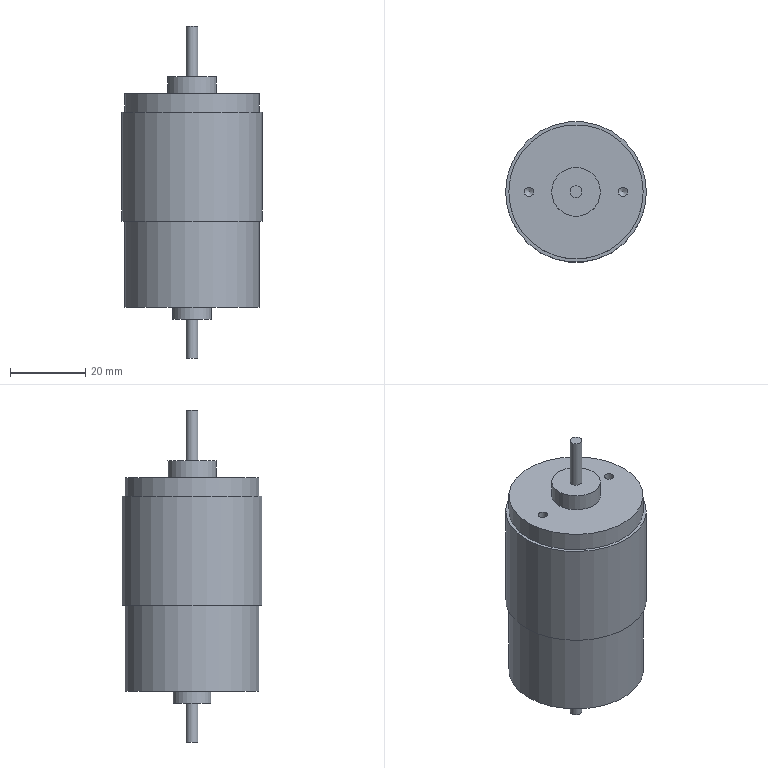Part | NX | features BREP 1, DATUM_CSYS 1 | 1 solid | 21 faces | box 37.5 x 37.5 x 88.5 mm | volume 61229 mm3 | cylinder 11 | plane 8 | cone 2 | commonest cylinder face diameters 2.5 x4 3.17 x2 35.8 x2 10.2 x1 13 x1 37.5 x1
STEP:
#1=CARTESIAN_POINT('',(17.9,0.,0.));
#2=VERTEX_POINT('',#1);
#3=CARTESIAN_POINT('',(0.,0.,0.));
#4=DIRECTION('',(0.,0.,1.));
#5=DIRECTION('',(1.,0.,0.));
#6=AXIS2_PLACEMENT_3D('',#3,#4,#5);
#7=CIRCLE('',#6,17.9);
#8=EDGE_CURVE('',#2,#2,#7,.T.);
#9=ORIENTED_EDGE('',*,*,#8,.F.);
#10=EDGE_LOOP('',(#9));
#11=FACE_BOUND('',#10,.T.);
#12=CARTESIAN_POINT('',(5.1,0.,0.));
#13=VERTEX_POINT('',#12);
#14=CARTESIAN_POINT('',(0.,0.,0.));
#15=DIRECTION('',(0.,0.,-1.));
#16=DIRECTION('',(1.,0.,0.));
#17=AXIS2_PLACEMENT_3D('',#14,#15,#16);
#18=CIRCLE('',#17,5.1);
#19=EDGE_CURVE('',#13,#13,#18,.T.);
#20=ORIENTED_EDGE('',*,*,#19,.F.);
#21=EDGE_LOOP('',(#20));
#22=FACE_BOUND('',#21,.T.);
#23=CARTESIAN_POINT('',(0.,0.,0.));
#24=DIRECTION('',(0.,0.,1.));
#25=DIRECTION('',(-1.,0.,0.));
#26=AXIS2_PLACEMENT_3D('',#23,#24,#25);
#27=PLANE('',#26);
#28=ADVANCED_FACE('',(#11,#22),#27,.F.);
#29=CARTESIAN_POINT('',(17.9,0.,57.));
#30=VERTEX_POINT('',#29);
#31=CARTESIAN_POINT('',(0.,0.,57.));
#32=DIRECTION('',(0.,0.,1.));
#33=DIRECTION('',(1.,0.,0.));
#34=AXIS2_PLACEMENT_3D('',#31,#32,#33);
#35=CIRCLE('',#34,17.9);
#36=EDGE_CURVE('',#30,#30,#35,.T.);
#37=ORIENTED_EDGE('',*,*,#36,.T.);
#38=EDGE_LOOP('',(#37));
#39=FACE_BOUND('',#38,.T.);
#40=CARTESIAN_POINT('',(6.5,0.,57.));
#41=VERTEX_POINT('',#40);
#42=CARTESIAN_POINT('',(0.,0.,57.));
#43=DIRECTION('',(0.,0.,1.));
#44=DIRECTION('',(1.,0.,0.));
#45=AXIS2_PLACEMENT_3D('',#42,#43,#44);
#46=CIRCLE('',#45,6.5);
#47=EDGE_CURVE('',#41,#41,#46,.T.);
#48=ORIENTED_EDGE('',*,*,#47,.F.);
#49=EDGE_LOOP('',(#48));
#50=FACE_BOUND('',#49,.T.);
#51=CARTESIAN_POINT('',(-11.25,0.,57.));
#52=VERTEX_POINT('',#51);
#53=CARTESIAN_POINT('',(-12.5,0.,57.));
#54=DIRECTION('',(0.,0.,-1.));
#55=DIRECTION('',(1.,0.,0.));
#56=AXIS2_PLACEMENT_3D('',#53,#54,#55);
#57=CIRCLE('',#56,1.25);
#58=EDGE_CURVE('',#52,#52,#57,.T.);
#59=ORIENTED_EDGE('',*,*,#58,.T.);
#60=EDGE_LOOP('',(#59));
#61=FACE_BOUND('',#60,.T.);
#62=CARTESIAN_POINT('',(13.75,0.,57.));
#63=VERTEX_POINT('',#62);
#64=CARTESIAN_POINT('',(12.5,0.,57.));
#65=DIRECTION('',(0.,0.,-1.));
#66=DIRECTION('',(1.,0.,0.));
#67=AXIS2_PLACEMENT_3D('',#64,#65,#66);
#68=CIRCLE('',#67,1.25);
#69=EDGE_CURVE('',#63,#63,#68,.T.);
#70=ORIENTED_EDGE('',*,*,#69,.T.);
#71=EDGE_LOOP('',(#70));
#72=FACE_BOUND('',#71,.T.);
#73=CARTESIAN_POINT('',(0.,0.,57.));
#74=DIRECTION('',(0.,0.,1.));
#75=DIRECTION('',(-1.,0.,0.));
#76=AXIS2_PLACEMENT_3D('',#73,#74,#75);
#77=PLANE('',#76);
#78=ADVANCED_FACE('',(#39,#50,#61,#72),#77,.T.);
#79=ORIENTED_EDGE('',*,*,#8,.T.);
#80=CARTESIAN_POINT('',(17.9,0.,23.));
#81=VERTEX_POINT('',#80);
#82=CARTESIAN_POINT('',(17.9,0.,0.));
#83=DIRECTION('',(0.,0.,1.));
#84=VECTOR('',#83,1000.);
#85=LINE('',#82,#84);
#86=EDGE_CURVE('',#2,#81,#85,.T.);
#87=ORIENTED_EDGE('',*,*,#86,.T.);
#88=CARTESIAN_POINT('',(0.,0.,23.));
#89=DIRECTION('',(0.,0.,1.));
#90=DIRECTION('',(1.,0.,0.));
#91=AXIS2_PLACEMENT_3D('',#88,#89,#90);
#92=CIRCLE('',#91,17.9);
#93=EDGE_CURVE('',#81,#81,#92,.T.);
#94=ORIENTED_EDGE('',*,*,#93,.F.);
#95=ORIENTED_EDGE('',*,*,#86,.F.);
#96=EDGE_LOOP('',(#79,#87,#94,#95));
#97=FACE_BOUND('',#96,.T.);
#98=CARTESIAN_POINT('',(0.,0.,0.));
#99=DIRECTION('',(0.,0.,1.));
#100=DIRECTION('',(-1.,0.,0.));
#101=AXIS2_PLACEMENT_3D('',#98,#99,#100);
#102=CYLINDRICAL_SURFACE('',#101,17.9);
#103=ADVANCED_FACE('',(#97),#102,.T.);
#104=ORIENTED_EDGE('',*,*,#36,.F.);
#105=CARTESIAN_POINT('',(17.9,0.,52.));
#106=VERTEX_POINT('',#105);
#107=CARTESIAN_POINT('',(17.9,0.,52.));
#108=DIRECTION('',(0.,0.,1.));
#109=VECTOR('',#108,1000.);
#110=LINE('',#107,#109);
#111=EDGE_CURVE('',#106,#30,#110,.T.);
#112=ORIENTED_EDGE('',*,*,#111,.F.);
#113=CARTESIAN_POINT('',(0.,0.,52.));
#114=DIRECTION('',(0.,0.,-1.));
#115=DIRECTION('',(1.,0.,0.));
#116=AXIS2_PLACEMENT_3D('',#113,#114,#115);
#117=CIRCLE('',#116,17.9);
#118=EDGE_CURVE('',#106,#106,#117,.T.);
#119=ORIENTED_EDGE('',*,*,#118,.F.);
#120=ORIENTED_EDGE('',*,*,#111,.T.);
#121=EDGE_LOOP('',(#104,#112,#119,#120));
#122=FACE_BOUND('',#121,.T.);
#123=CARTESIAN_POINT('',(0.,0.,0.));
#124=DIRECTION('',(0.,0.,1.));
#125=DIRECTION('',(-1.,0.,0.));
#126=AXIS2_PLACEMENT_3D('',#123,#124,#125);
#127=CYLINDRICAL_SURFACE('',#126,17.9);
#128=ADVANCED_FACE('',(#122),#127,.T.);
#129=CARTESIAN_POINT('',(18.75,0.,23.));
#130=VERTEX_POINT('',#129);
#131=CARTESIAN_POINT('',(0.,0.,23.));
#132=DIRECTION('',(0.,0.,1.));
#133=DIRECTION('',(1.,0.,0.));
#134=AXIS2_PLACEMENT_3D('',#131,#132,#133);
#135=CIRCLE('',#134,18.75);
#136=EDGE_CURVE('',#130,#130,#135,.T.);
#137=ORIENTED_EDGE('',*,*,#136,.F.);
#138=EDGE_LOOP('',(#137));
#139=FACE_BOUND('',#138,.T.);
#140=ORIENTED_EDGE('',*,*,#93,.T.);
#141=EDGE_LOOP('',(#140));
#142=FACE_BOUND('',#141,.T.);
#143=CARTESIAN_POINT('',(-5.024,0.,23.));
#144=DIRECTION('',(0.,0.,1.));
#145=DIRECTION('',(-1.,0.,0.));
#146=AXIS2_PLACEMENT_3D('',#143,#144,#145);
#147=PLANE('',#146);
#148=ADVANCED_FACE('',(#139,#142),#147,.F.);
#149=CARTESIAN_POINT('',(18.75,0.,52.));
#150=VERTEX_POINT('',#149);
#151=CARTESIAN_POINT('',(18.75,0.,52.));
#152=DIRECTION('',(0.,0.,-1.));
#153=VECTOR('',#152,1000.);
#154=LINE('',#151,#153);
#155=EDGE_CURVE('',#150,#130,#154,.T.);
#156=ORIENTED_EDGE('',*,*,#155,.T.);
#157=ORIENTED_EDGE('',*,*,#136,.T.);
#158=ORIENTED_EDGE('',*,*,#155,.F.);
#159=CARTESIAN_POINT('',(0.,0.,52.));
#160=DIRECTION('',(0.,0.,1.));
#161=DIRECTION('',(1.,0.,0.));
#162=AXIS2_PLACEMENT_3D('',#159,#160,#161);
#163=CIRCLE('',#162,18.75);
#164=EDGE_CURVE('',#150,#150,#163,.T.);
#165=ORIENTED_EDGE('',*,*,#164,.F.);
#166=EDGE_LOOP('',(#156,#157,#158,#165));
#167=FACE_BOUND('',#166,.T.);
#168=CARTESIAN_POINT('',(0.,0.,52.));
#169=DIRECTION('',(0.,0.,-1.));
#170=DIRECTION('',(-1.,0.,0.));
#171=AXIS2_PLACEMENT_3D('',#168,#169,#170);
#172=CYLINDRICAL_SURFACE('',#171,18.75);
#173=ADVANCED_FACE('',(#167),#172,.T.);
#174=ORIENTED_EDGE('',*,*,#164,.T.);
#175=EDGE_LOOP('',(#174));
#176=FACE_BOUND('',#175,.T.);
#177=ORIENTED_EDGE('',*,*,#118,.T.);
#178=EDGE_LOOP('',(#177));
#179=FACE_BOUND('',#178,.T.);
#180=CARTESIAN_POINT('',(-5.024,0.,52.));
#181=DIRECTION('',(0.,0.,1.));
#182=DIRECTION('',(-1.,0.,0.));
#183=AXIS2_PLACEMENT_3D('',#180,#181,#182);
#184=PLANE('',#183);
#185=ADVANCED_FACE('',(#176,#179),#184,.T.);
#186=ORIENTED_EDGE('',*,*,#19,.T.);
#187=CARTESIAN_POINT('',(5.1,0.,-3.2));
#188=VERTEX_POINT('',#187);
#189=CARTESIAN_POINT('',(5.1,0.,0.));
#190=DIRECTION('',(0.,0.,-1.));
#191=VECTOR('',#190,1000.);
#192=LINE('',#189,#191);
#193=EDGE_CURVE('',#13,#188,#192,.T.);
#194=ORIENTED_EDGE('',*,*,#193,.T.);
#195=CARTESIAN_POINT('',(0.,0.,-3.2));
#196=DIRECTION('',(0.,0.,-1.));
#197=DIRECTION('',(1.,0.,0.));
#198=AXIS2_PLACEMENT_3D('',#195,#196,#197);
#199=CIRCLE('',#198,5.1);
#200=EDGE_CURVE('',#188,#188,#199,.T.);
#201=ORIENTED_EDGE('',*,*,#200,.F.);
#202=ORIENTED_EDGE('',*,*,#193,.F.);
#203=EDGE_LOOP('',(#186,#194,#201,#202));
#204=FACE_BOUND('',#203,.T.);
#205=CARTESIAN_POINT('',(0.,0.,0.));
#206=DIRECTION('',(0.,0.,-1.));
#207=DIRECTION('',(-1.,0.,0.));
#208=AXIS2_PLACEMENT_3D('',#205,#206,#207);
#209=CYLINDRICAL_SURFACE('',#208,5.1);
#210=ADVANCED_FACE('',(#204),#209,.T.);
#211=ORIENTED_EDGE('',*,*,#200,.T.);
#212=EDGE_LOOP('',(#211));
#213=FACE_BOUND('',#212,.T.);
#214=CARTESIAN_POINT('',(1.585,0.,-3.2));
#215=VERTEX_POINT('',#214);
#216=CARTESIAN_POINT('',(0.,0.,-3.2));
#217=DIRECTION('',(0.,0.,-1.));
#218=DIRECTION('',(1.,0.,0.));
#219=AXIS2_PLACEMENT_3D('',#216,#217,#218);
#220=CIRCLE('',#219,1.585);
#221=EDGE_CURVE('',#215,#215,#220,.T.);
#222=ORIENTED_EDGE('',*,*,#221,.F.);
#223=EDGE_LOOP('',(#222));
#224=FACE_BOUND('',#223,.T.);
#225=CARTESIAN_POINT('',(0.,0.,-3.2));
#226=DIRECTION('',(0.,0.,-1.));
#227=DIRECTION('',(-1.,0.,0.));
#228=AXIS2_PLACEMENT_3D('',#225,#226,#227);
#229=PLANE('',#228);
#230=ADVANCED_FACE('',(#213,#224),#229,.T.);
#231=ORIENTED_EDGE('',*,*,#221,.T.);
#232=CARTESIAN_POINT('',(1.585,0.,-13.5));
#233=VERTEX_POINT('',#232);
#234=CARTESIAN_POINT('',(1.585,0.,-3.2));
#235=DIRECTION('',(0.,0.,-1.));
#236=VECTOR('',#235,1000.);
#237=LINE('',#234,#236);
#238=EDGE_CURVE('',#215,#233,#237,.T.);
#239=ORIENTED_EDGE('',*,*,#238,.T.);
#240=CARTESIAN_POINT('',(0.,0.,-13.5));
#241=DIRECTION('',(0.,0.,-1.));
#242=DIRECTION('',(1.,0.,0.));
#243=AXIS2_PLACEMENT_3D('',#240,#241,#242);
#244=CIRCLE('',#243,1.585);
#245=EDGE_CURVE('',#233,#233,#244,.T.);
#246=ORIENTED_EDGE('',*,*,#245,.F.);
#247=ORIENTED_EDGE('',*,*,#238,.F.);
#248=EDGE_LOOP('',(#231,#239,#246,#247));
#249=FACE_BOUND('',#248,.T.);
#250=CARTESIAN_POINT('',(0.,0.,-3.2));
#251=DIRECTION('',(0.,0.,-1.));
#252=DIRECTION('',(-1.,0.,0.));
#253=AXIS2_PLACEMENT_3D('',#250,#251,#252);
#254=CYLINDRICAL_SURFACE('',#253,1.585);
#255=ADVANCED_FACE('',(#249),#254,.T.);
#256=ORIENTED_EDGE('',*,*,#245,.T.);
#257=EDGE_LOOP('',(#256));
#258=FACE_BOUND('',#257,.T.);
#259=CARTESIAN_POINT('',(0.,0.,-13.5));
#260=DIRECTION('',(0.,0.,-1.));
#261=DIRECTION('',(-1.,0.,0.));
#262=AXIS2_PLACEMENT_3D('',#259,#260,#261);
#263=PLANE('',#262);
#264=ADVANCED_FACE('',(#258),#263,.T.);
#265=ORIENTED_EDGE('',*,*,#47,.T.);
#266=CARTESIAN_POINT('',(6.5,0.,61.5));
#267=VERTEX_POINT('',#266);
#268=CARTESIAN_POINT('',(6.5,0.,57.));
#269=DIRECTION('',(0.,0.,1.));
#270=VECTOR('',#269,1000.);
#271=LINE('',#268,#270);
#272=EDGE_CURVE('',#41,#267,#271,.T.);
#273=ORIENTED_EDGE('',*,*,#272,.T.);
#274=CARTESIAN_POINT('',(0.,0.,61.5));
#275=DIRECTION('',(0.,0.,1.));
#276=DIRECTION('',(1.,0.,0.));
#277=AXIS2_PLACEMENT_3D('',#274,#275,#276);
#278=CIRCLE('',#277,6.5);
#279=EDGE_CURVE('',#267,#267,#278,.T.);
#280=ORIENTED_EDGE('',*,*,#279,.F.);
#281=ORIENTED_EDGE('',*,*,#272,.F.);
#282=EDGE_LOOP('',(#265,#273,#280,#281));
#283=FACE_BOUND('',#282,.T.);
#284=CARTESIAN_POINT('',(0.,0.,57.));
#285=DIRECTION('',(0.,0.,1.));
#286=DIRECTION('',(-1.,0.,0.));
#287=AXIS2_PLACEMENT_3D('',#284,#285,#286);
#288=CYLINDRICAL_SURFACE('',#287,6.5);
#289=ADVANCED_FACE('',(#283),#288,.T.);
#290=ORIENTED_EDGE('',*,*,#279,.T.);
#291=EDGE_LOOP('',(#290));
#292=FACE_BOUND('',#291,.T.);
#293=CARTESIAN_POINT('',(1.585,0.,61.5));
#294=VERTEX_POINT('',#293);
#295=CARTESIAN_POINT('',(0.,0.,61.5));
#296=DIRECTION('',(0.,0.,1.));
#297=DIRECTION('',(1.,0.,0.));
#298=AXIS2_PLACEMENT_3D('',#295,#296,#297);
#299=CIRCLE('',#298,1.585);
#300=EDGE_CURVE('',#294,#294,#299,.T.);
#301=ORIENTED_EDGE('',*,*,#300,.F.);
#302=EDGE_LOOP('',(#301));
#303=FACE_BOUND('',#302,.T.);
#304=CARTESIAN_POINT('',(0.,0.,61.5));
#305=DIRECTION('',(0.,0.,1.));
#306=DIRECTION('',(-1.,0.,0.));
#307=AXIS2_PLACEMENT_3D('',#304,#305,#306);
#308=PLANE('',#307);
#309=ADVANCED_FACE('',(#292,#303),#308,.T.);
#310=ORIENTED_EDGE('',*,*,#300,.T.);
#311=CARTESIAN_POINT('',(1.585,0.,75.));
#312=VERTEX_POINT('',#311);
#313=CARTESIAN_POINT('',(1.585,0.,61.5));
#314=DIRECTION('',(0.,0.,1.));
#315=VECTOR('',#314,1000.);
#316=LINE('',#313,#315);
#317=EDGE_CURVE('',#294,#312,#316,.T.);
#318=ORIENTED_EDGE('',*,*,#317,.T.);
#319=CARTESIAN_POINT('',(0.,0.,75.));
#320=DIRECTION('',(0.,0.,1.));
#321=DIRECTION('',(1.,0.,0.));
#322=AXIS2_PLACEMENT_3D('',#319,#320,#321);
#323=CIRCLE('',#322,1.585);
#324=EDGE_CURVE('',#312,#312,#323,.T.);
#325=ORIENTED_EDGE('',*,*,#324,.F.);
#326=ORIENTED_EDGE('',*,*,#317,.F.);
#327=EDGE_LOOP('',(#310,#318,#325,#326));
#328=FACE_BOUND('',#327,.T.);
#329=CARTESIAN_POINT('',(0.,0.,61.5));
#330=DIRECTION('',(0.,0.,1.));
#331=DIRECTION('',(-1.,0.,0.));
#332=AXIS2_PLACEMENT_3D('',#329,#330,#331);
#333=CYLINDRICAL_SURFACE('',#332,1.585);
#334=ADVANCED_FACE('',(#328),#333,.T.);
#335=ORIENTED_EDGE('',*,*,#324,.T.);
#336=EDGE_LOOP('',(#335));
#337=FACE_BOUND('',#336,.T.);
#338=CARTESIAN_POINT('',(0.,0.,75.));
#339=DIRECTION('',(0.,0.,1.));
#340=DIRECTION('',(-1.,0.,0.));
#341=AXIS2_PLACEMENT_3D('',#338,#339,#340);
#342=PLANE('',#341);
#343=ADVANCED_FACE('',(#337),#342,.T.);
#344=CARTESIAN_POINT('',(-11.25,0.,55.));
#345=VERTEX_POINT('',#344);
#346=CARTESIAN_POINT('',(-11.25,0.,57.));
#347=DIRECTION('',(0.,0.,-1.));
#348=VECTOR('',#347,1000.);
#349=LINE('',#346,#348);
#350=EDGE_CURVE('',#52,#345,#349,.T.);
#351=ORIENTED_EDGE('',*,*,#350,.T.);
#352=CARTESIAN_POINT('',(-12.5,0.,55.));
#353=DIRECTION('',(0.,0.,-1.));
#354=DIRECTION('',(1.,0.,0.));
#355=AXIS2_PLACEMENT_3D('',#352,#353,#354);
#356=CIRCLE('',#355,1.25);
#357=EDGE_CURVE('',#345,#345,#356,.T.);
#358=ORIENTED_EDGE('',*,*,#357,.T.);
#359=ORIENTED_EDGE('',*,*,#350,.F.);
#360=ORIENTED_EDGE('',*,*,#58,.F.);
#361=EDGE_LOOP('',(#351,#358,#359,#360));
#362=FACE_BOUND('',#361,.T.);
#363=CARTESIAN_POINT('',(-12.5,0.,57.));
#364=DIRECTION('',(0.,0.,-1.));
#365=DIRECTION('',(-1.,0.,0.));
#366=AXIS2_PLACEMENT_3D('',#363,#364,#365);
#367=CYLINDRICAL_SURFACE('',#366,1.25);
#368=ADVANCED_FACE('',(#362),#367,.F.);
#369=CARTESIAN_POINT('',(13.75,0.,55.));
#370=VERTEX_POINT('',#369);
#371=CARTESIAN_POINT('',(13.75,0.,57.));
#372=DIRECTION('',(0.,0.,-1.));
#373=VECTOR('',#372,1000.);
#374=LINE('',#371,#373);
#375=EDGE_CURVE('',#63,#370,#374,.T.);
#376=ORIENTED_EDGE('',*,*,#375,.T.);
#377=CARTESIAN_POINT('',(12.5,0.,55.));
#378=DIRECTION('',(0.,0.,-1.));
#379=DIRECTION('',(1.,0.,0.));
#380=AXIS2_PLACEMENT_3D('',#377,#378,#379);
#381=CIRCLE('',#380,1.25);
#382=EDGE_CURVE('',#370,#370,#381,.T.);
#383=ORIENTED_EDGE('',*,*,#382,.T.);
#384=ORIENTED_EDGE('',*,*,#375,.F.);
#385=ORIENTED_EDGE('',*,*,#69,.F.);
#386=EDGE_LOOP('',(#376,#383,#384,#385));
#387=FACE_BOUND('',#386,.T.);
#388=CARTESIAN_POINT('',(12.5,0.,57.));
#389=DIRECTION('',(0.,0.,-1.));
#390=DIRECTION('',(-1.,0.,0.));
#391=AXIS2_PLACEMENT_3D('',#388,#389,#390);
#392=CYLINDRICAL_SURFACE('',#391,1.25);
#393=ADVANCED_FACE('',(#387),#392,.F.);
#394=CARTESIAN_POINT('',(-11.25,0.,54.));
#395=VERTEX_POINT('',#394);
#396=CARTESIAN_POINT('',(-11.25,0.,55.));
#397=DIRECTION('',(0.,0.,-1.));
#398=VECTOR('',#397,1000.);
#399=LINE('',#396,#398);
#400=EDGE_CURVE('',#345,#395,#399,.T.);
#401=ORIENTED_EDGE('',*,*,#400,.T.);
#402=CARTESIAN_POINT('',(-12.5,0.,54.));
#403=DIRECTION('',(0.,0.,-1.));
#404=DIRECTION('',(1.,0.,0.));
#405=AXIS2_PLACEMENT_3D('',#402,#403,#404);
#406=CIRCLE('',#405,1.25);
#407=EDGE_CURVE('',#395,#395,#406,.T.);
#408=ORIENTED_EDGE('',*,*,#407,.T.);
#409=ORIENTED_EDGE('',*,*,#400,.F.);
#410=ORIENTED_EDGE('',*,*,#357,.F.);
#411=EDGE_LOOP('',(#401,#408,#409,#410));
#412=FACE_BOUND('',#411,.T.);
#413=CARTESIAN_POINT('',(-12.5,0.,55.));
#414=DIRECTION('',(0.,0.,-1.));
#415=DIRECTION('',(-1.,0.,0.));
#416=AXIS2_PLACEMENT_3D('',#413,#414,#415);
#417=CYLINDRICAL_SURFACE('',#416,1.25);
#418=ADVANCED_FACE('',(#412),#417,.F.);
#419=CARTESIAN_POINT('',(13.75,0.,54.));
#420=VERTEX_POINT('',#419);
#421=CARTESIAN_POINT('',(13.75,0.,55.));
#422=DIRECTION('',(0.,0.,-1.));
#423=VECTOR('',#422,1000.);
#424=LINE('',#421,#423);
#425=EDGE_CURVE('',#370,#420,#424,.T.);
#426=ORIENTED_EDGE('',*,*,#425,.T.);
#427=CARTESIAN_POINT('',(12.5,0.,54.));
#428=DIRECTION('',(0.,0.,-1.));
#429=DIRECTION('',(1.,0.,0.));
#430=AXIS2_PLACEMENT_3D('',#427,#428,#429);
#431=CIRCLE('',#430,1.25);
#432=EDGE_CURVE('',#420,#420,#431,.T.);
#433=ORIENTED_EDGE('',*,*,#432,.T.);
#434=ORIENTED_EDGE('',*,*,#425,.F.);
#435=ORIENTED_EDGE('',*,*,#382,.F.);
#436=EDGE_LOOP('',(#426,#433,#434,#435));
#437=FACE_BOUND('',#436,.T.);
#438=CARTESIAN_POINT('',(12.5,0.,55.));
#439=DIRECTION('',(0.,0.,-1.));
#440=DIRECTION('',(-1.,0.,0.));
#441=AXIS2_PLACEMENT_3D('',#438,#439,#440);
#442=CYLINDRICAL_SURFACE('',#441,1.25);
#443=ADVANCED_FACE('',(#437),#442,.F.);
#444=CARTESIAN_POINT('',(-12.5,0.,53.249));
#445=VERTEX_POINT('',#444);
#446=CARTESIAN_POINT('',(-11.25,0.,54.));
#447=DIRECTION('',(-0.8572,0.,-0.515));
#448=VECTOR('',#447,1000.);
#449=LINE('',#446,#448);
#450=EDGE_CURVE('',#395,#445,#449,.T.);
#451=ORIENTED_EDGE('',*,*,#450,.T.);
#452=ORIENTED_EDGE('',*,*,#450,.F.);
#453=ORIENTED_EDGE('',*,*,#407,.F.);
#454=EDGE_LOOP('',(#451,#452,#453));
#455=FACE_BOUND('',#454,.T.);
#456=CARTESIAN_POINT('',(-12.5,0.,53.249));
#457=DIRECTION('',(0.,0.,1.));
#458=DIRECTION('',(-1.,0.,0.));
#459=AXIS2_PLACEMENT_3D('',#456,#457,#458);
#460=CONICAL_SURFACE('',#459,0.,1.03);
#461=ADVANCED_FACE('',(#455),#460,.F.);
#462=CARTESIAN_POINT('',(12.5,0.,53.249));
#463=VERTEX_POINT('',#462);
#464=CARTESIAN_POINT('',(13.75,0.,54.));
#465=DIRECTION('',(-0.8572,0.,-0.515));
#466=VECTOR('',#465,1000.);
#467=LINE('',#464,#466);
#468=EDGE_CURVE('',#420,#463,#467,.T.);
#469=ORIENTED_EDGE('',*,*,#468,.T.);
#470=ORIENTED_EDGE('',*,*,#468,.F.);
#471=ORIENTED_EDGE('',*,*,#432,.F.);
#472=EDGE_LOOP('',(#469,#470,#471));
#473=FACE_BOUND('',#472,.T.);
#474=CARTESIAN_POINT('',(12.5,0.,53.249));
#475=DIRECTION('',(0.,0.,1.));
#476=DIRECTION('',(-1.,0.,0.));
#477=AXIS2_PLACEMENT_3D('',#474,#475,#476);
#478=CONICAL_SURFACE('',#477,0.,1.03);
#479=ADVANCED_FACE('',(#473),#478,.F.);
#480=CLOSED_SHELL('',(#28,#78,#103,#128,#148,#173,#185,#210,#230,#255,#264,#289,#309,#334,#343,#368,#393,#418,#443,#461,#479));
#481=MANIFOLD_SOLID_BREP('',#480);
#482=(LENGTH_UNIT()NAMED_UNIT(*)SI_UNIT(.MILLI.,.METRE.));
#483=UNCERTAINTY_MEASURE_WITH_UNIT(LENGTH_MEASURE(0.00001),#482,'','');
#484=(NAMED_UNIT(*)PLANE_ANGLE_UNIT()SI_UNIT($,.RADIAN.));
#485=(NAMED_UNIT(*)SI_UNIT($,.STERADIAN.)SOLID_ANGLE_UNIT());
#486=(GEOMETRIC_REPRESENTATION_CONTEXT(3)GLOBAL_UNCERTAINTY_ASSIGNED_CONTEXT((#483))GLOBAL_UNIT_ASSIGNED_CONTEXT((#482,#484,#485))REPRESENTATION_CONTEXT('',''));
#487=ADVANCED_BREP_SHAPE_REPRESENTATION('',(#481),#486);